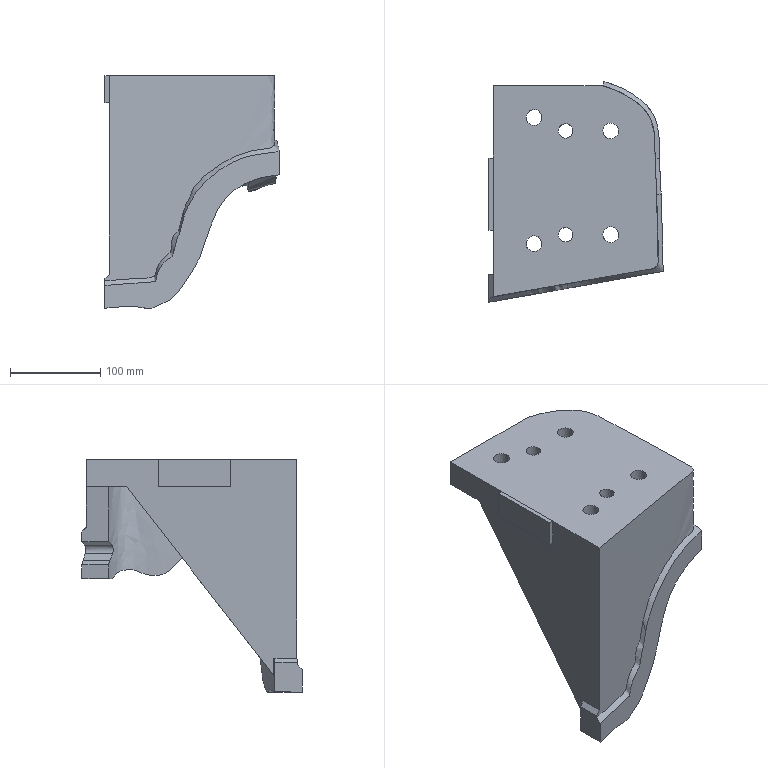Part | NX | features solid 2 | 1 solid | 51 faces | box 193.881 x 244.158 x 258.143 mm | volume 2759639 mm3 | plane 23 | spline 17 | cylinder 11 | commonest cylinder face diameters 17.5 x4 25 x4 16 x2 12 x1